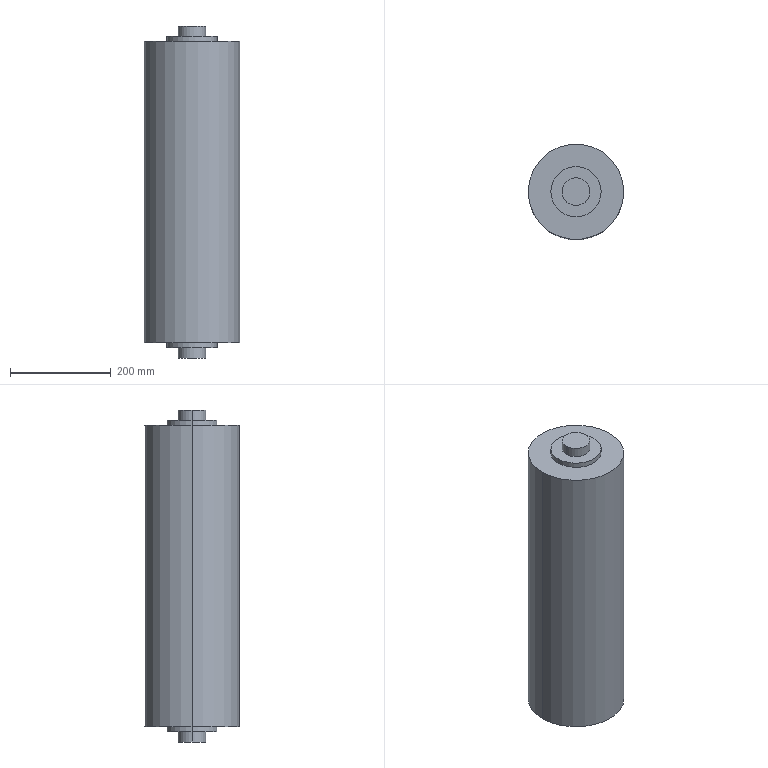Part | SolidWorks | features ICE 4, Extrusion 1 | 1 solid | 16 faces | box 190 x 190 x 660 mm | volume 17263837 mm3 | cylinder 10 | plane 6 | commonest cylinder face diameters 55 x4 100 x4 190 x2
STEP:
#1=CARTESIAN_POINT('',(27.5,0.,630.));
#2=VERTEX_POINT('',#1);
#3=CARTESIAN_POINT('',(-27.5,0.,630.));
#4=VERTEX_POINT('',#3);
#5=CARTESIAN_POINT('',(0.,0.,630.));
#6=DIRECTION('',(0.,0.,1.));
#7=DIRECTION('',(1.,0.,0.));
#8=AXIS2_PLACEMENT_3D('',#5,#6,#7);
#9=CIRCLE('',#8,27.5);
#10=EDGE_CURVE('',#2,#4,#9,.T.);
#11=ORIENTED_EDGE('',*,*,#10,.F.);
#12=CARTESIAN_POINT('',(27.5,0.,610.));
#13=VERTEX_POINT('',#12);
#14=CARTESIAN_POINT('',(27.5,0.,630.));
#15=DIRECTION('',(0.,0.,-1.));
#16=VECTOR('',#15,1000.);
#17=LINE('',#14,#16);
#18=EDGE_CURVE('',#2,#13,#17,.T.);
#19=ORIENTED_EDGE('',*,*,#18,.T.);
#20=CARTESIAN_POINT('',(-27.5,0.,610.));
#21=VERTEX_POINT('',#20);
#22=CARTESIAN_POINT('',(0.,0.,610.));
#23=DIRECTION('',(0.,0.,1.));
#24=DIRECTION('',(1.,0.,0.));
#25=AXIS2_PLACEMENT_3D('',#22,#23,#24);
#26=CIRCLE('',#25,27.5);
#27=EDGE_CURVE('',#13,#21,#26,.T.);
#28=ORIENTED_EDGE('',*,*,#27,.T.);
#29=CARTESIAN_POINT('',(-27.5,0.,630.));
#30=DIRECTION('',(0.,0.,-1.));
#31=VECTOR('',#30,1000.);
#32=LINE('',#29,#31);
#33=EDGE_CURVE('',#4,#21,#32,.T.);
#34=ORIENTED_EDGE('',*,*,#33,.F.);
#35=EDGE_LOOP('',(#11,#19,#28,#34));
#36=FACE_OUTER_BOUND('',#35,.T.);
#37=CARTESIAN_POINT('',(0.,0.,630.));
#38=DIRECTION('',(0.,0.,-1.));
#39=DIRECTION('',(-1.,0.,0.));
#40=AXIS2_PLACEMENT_3D('',#37,#38,#39);
#41=CYLINDRICAL_SURFACE('',#40,27.5);
#42=ADVANCED_FACE('',(#36),#41,.T.);
#43=CARTESIAN_POINT('',(-27.5,0.,-30.));
#44=VERTEX_POINT('',#43);
#45=CARTESIAN_POINT('',(27.5,0.,-30.));
#46=VERTEX_POINT('',#45);
#47=CARTESIAN_POINT('',(0.,0.,-30.));
#48=DIRECTION('',(0.,0.,-1.));
#49=DIRECTION('',(-1.,0.,0.));
#50=AXIS2_PLACEMENT_3D('',#47,#48,#49);
#51=CIRCLE('',#50,27.5);
#52=EDGE_CURVE('',#44,#46,#51,.T.);
#53=ORIENTED_EDGE('',*,*,#52,.F.);
#54=CARTESIAN_POINT('',(-27.5,0.,-10.));
#55=VERTEX_POINT('',#54);
#56=CARTESIAN_POINT('',(-27.5,0.,-30.));
#57=DIRECTION('',(0.,0.,1.));
#58=VECTOR('',#57,1000.);
#59=LINE('',#56,#58);
#60=EDGE_CURVE('',#44,#55,#59,.T.);
#61=ORIENTED_EDGE('',*,*,#60,.T.);
#62=CARTESIAN_POINT('',(27.5,0.,-10.));
#63=VERTEX_POINT('',#62);
#64=CARTESIAN_POINT('',(0.,0.,-10.));
#65=DIRECTION('',(0.,0.,-1.));
#66=DIRECTION('',(-1.,0.,0.));
#67=AXIS2_PLACEMENT_3D('',#64,#65,#66);
#68=CIRCLE('',#67,27.5);
#69=EDGE_CURVE('',#55,#63,#68,.T.);
#70=ORIENTED_EDGE('',*,*,#69,.T.);
#71=CARTESIAN_POINT('',(27.5,0.,-30.));
#72=DIRECTION('',(0.,0.,1.));
#73=VECTOR('',#72,1000.);
#74=LINE('',#71,#73);
#75=EDGE_CURVE('',#46,#63,#74,.T.);
#76=ORIENTED_EDGE('',*,*,#75,.F.);
#77=EDGE_LOOP('',(#53,#61,#70,#76));
#78=FACE_OUTER_BOUND('',#77,.T.);
#79=CARTESIAN_POINT('',(0.,0.,-30.));
#80=DIRECTION('',(0.,0.,1.));
#81=DIRECTION('',(1.,0.,0.));
#82=AXIS2_PLACEMENT_3D('',#79,#80,#81);
#83=CYLINDRICAL_SURFACE('',#82,27.5);
#84=ADVANCED_FACE('',(#78),#83,.T.);
#85=CARTESIAN_POINT('',(-50.,0.,-10.));
#86=VERTEX_POINT('',#85);
#87=CARTESIAN_POINT('',(50.,0.,-10.));
#88=VERTEX_POINT('',#87);
#89=CARTESIAN_POINT('',(0.,0.,-10.));
#90=DIRECTION('',(0.,0.,-1.));
#91=DIRECTION('',(-1.,0.,0.));
#92=AXIS2_PLACEMENT_3D('',#89,#90,#91);
#93=CIRCLE('',#92,50.);
#94=EDGE_CURVE('',#86,#88,#93,.T.);
#95=ORIENTED_EDGE('',*,*,#94,.F.);
#96=CARTESIAN_POINT('',(-50.,0.,0.));
#97=VERTEX_POINT('',#96);
#98=CARTESIAN_POINT('',(-50.,0.,-10.));
#99=DIRECTION('',(0.,0.,1.));
#100=VECTOR('',#99,1000.);
#101=LINE('',#98,#100);
#102=EDGE_CURVE('',#86,#97,#101,.T.);
#103=ORIENTED_EDGE('',*,*,#102,.T.);
#104=CARTESIAN_POINT('',(50.,0.,0.));
#105=VERTEX_POINT('',#104);
#106=CARTESIAN_POINT('',(0.,0.,0.));
#107=DIRECTION('',(0.,0.,-1.));
#108=DIRECTION('',(1.,0.,0.));
#109=AXIS2_PLACEMENT_3D('',#106,#107,#108);
#110=CIRCLE('',#109,50.);
#111=EDGE_CURVE('',#97,#105,#110,.T.);
#112=ORIENTED_EDGE('',*,*,#111,.T.);
#113=CARTESIAN_POINT('',(50.,0.,-10.));
#114=DIRECTION('',(0.,0.,1.));
#115=VECTOR('',#114,1000.);
#116=LINE('',#113,#115);
#117=EDGE_CURVE('',#88,#105,#116,.T.);
#118=ORIENTED_EDGE('',*,*,#117,.F.);
#119=EDGE_LOOP('',(#95,#103,#112,#118));
#120=FACE_OUTER_BOUND('',#119,.T.);
#121=CARTESIAN_POINT('',(0.,0.,-10.));
#122=DIRECTION('',(0.,0.,1.));
#123=DIRECTION('',(1.,0.,0.));
#124=AXIS2_PLACEMENT_3D('',#121,#122,#123);
#125=CYLINDRICAL_SURFACE('',#124,50.);
#126=ADVANCED_FACE('',(#120),#125,.T.);
#127=CARTESIAN_POINT('',(50.,0.,610.));
#128=VERTEX_POINT('',#127);
#129=CARTESIAN_POINT('',(-50.,0.,610.));
#130=VERTEX_POINT('',#129);
#131=CARTESIAN_POINT('',(0.,0.,610.));
#132=DIRECTION('',(0.,0.,1.));
#133=DIRECTION('',(1.,0.,0.));
#134=AXIS2_PLACEMENT_3D('',#131,#132,#133);
#135=CIRCLE('',#134,50.);
#136=EDGE_CURVE('',#128,#130,#135,.T.);
#137=ORIENTED_EDGE('',*,*,#136,.F.);
#138=CARTESIAN_POINT('',(50.,0.,600.));
#139=VERTEX_POINT('',#138);
#140=CARTESIAN_POINT('',(50.,0.,610.));
#141=DIRECTION('',(0.,0.,-1.));
#142=VECTOR('',#141,1000.);
#143=LINE('',#140,#142);
#144=EDGE_CURVE('',#128,#139,#143,.T.);
#145=ORIENTED_EDGE('',*,*,#144,.T.);
#146=CARTESIAN_POINT('',(-50.,0.,600.));
#147=VERTEX_POINT('',#146);
#148=CARTESIAN_POINT('',(0.,0.,600.));
#149=DIRECTION('',(0.,0.,1.));
#150=DIRECTION('',(1.,0.,0.));
#151=AXIS2_PLACEMENT_3D('',#148,#149,#150);
#152=CIRCLE('',#151,50.);
#153=EDGE_CURVE('',#139,#147,#152,.T.);
#154=ORIENTED_EDGE('',*,*,#153,.T.);
#155=CARTESIAN_POINT('',(-50.,0.,610.));
#156=DIRECTION('',(0.,0.,-1.));
#157=VECTOR('',#156,1000.);
#158=LINE('',#155,#157);
#159=EDGE_CURVE('',#130,#147,#158,.T.);
#160=ORIENTED_EDGE('',*,*,#159,.F.);
#161=EDGE_LOOP('',(#137,#145,#154,#160));
#162=FACE_OUTER_BOUND('',#161,.T.);
#163=CARTESIAN_POINT('',(0.,0.,610.));
#164=DIRECTION('',(0.,0.,-1.));
#165=DIRECTION('',(-1.,0.,0.));
#166=AXIS2_PLACEMENT_3D('',#163,#164,#165);
#167=CYLINDRICAL_SURFACE('',#166,50.);
#168=ADVANCED_FACE('',(#162),#167,.T.);
#169=CARTESIAN_POINT('',(95.,0.,600.));
#170=VERTEX_POINT('',#169);
#171=CARTESIAN_POINT('',(-95.,0.,600.));
#172=VERTEX_POINT('',#171);
#173=CARTESIAN_POINT('',(0.,0.,600.));
#174=DIRECTION('',(0.,0.,1.));
#175=DIRECTION('',(1.,0.,0.));
#176=AXIS2_PLACEMENT_3D('',#173,#174,#175);
#177=CIRCLE('',#176,95.);
#178=EDGE_CURVE('',#170,#172,#177,.T.);
#179=ORIENTED_EDGE('',*,*,#178,.F.);
#180=CARTESIAN_POINT('',(95.,0.,0.));
#181=VERTEX_POINT('',#180);
#182=CARTESIAN_POINT('',(95.,0.,600.));
#183=DIRECTION('',(0.,0.,-1.));
#184=VECTOR('',#183,1000.);
#185=LINE('',#182,#184);
#186=EDGE_CURVE('',#170,#181,#185,.T.);
#187=ORIENTED_EDGE('',*,*,#186,.T.);
#188=CARTESIAN_POINT('',(-95.,0.,0.));
#189=VERTEX_POINT('',#188);
#190=CARTESIAN_POINT('',(0.,0.,0.));
#191=DIRECTION('',(0.,0.,1.));
#192=DIRECTION('',(1.,0.,0.));
#193=AXIS2_PLACEMENT_3D('',#190,#191,#192);
#194=CIRCLE('',#193,95.);
#195=EDGE_CURVE('',#181,#189,#194,.T.);
#196=ORIENTED_EDGE('',*,*,#195,.T.);
#197=CARTESIAN_POINT('',(-95.,0.,600.));
#198=DIRECTION('',(0.,0.,-1.));
#199=VECTOR('',#198,1000.);
#200=LINE('',#197,#199);
#201=EDGE_CURVE('',#172,#189,#200,.T.);
#202=ORIENTED_EDGE('',*,*,#201,.F.);
#203=EDGE_LOOP('',(#179,#187,#196,#202));
#204=FACE_OUTER_BOUND('',#203,.T.);
#205=CARTESIAN_POINT('',(0.,0.,600.));
#206=DIRECTION('',(0.,0.,-1.));
#207=DIRECTION('',(-1.,0.,0.));
#208=AXIS2_PLACEMENT_3D('',#205,#206,#207);
#209=CYLINDRICAL_SURFACE('',#208,95.);
#210=ADVANCED_FACE('',(#204),#209,.T.);
#211=ORIENTED_EDGE('',*,*,#186,.F.);
#212=CARTESIAN_POINT('',(0.,0.,600.));
#213=DIRECTION('',(0.,0.,1.));
#214=DIRECTION('',(1.,0.,0.));
#215=AXIS2_PLACEMENT_3D('',#212,#213,#214);
#216=CIRCLE('',#215,95.);
#217=EDGE_CURVE('',#172,#170,#216,.T.);
#218=ORIENTED_EDGE('',*,*,#217,.F.);
#219=ORIENTED_EDGE('',*,*,#201,.T.);
#220=CARTESIAN_POINT('',(0.,0.,0.));
#221=DIRECTION('',(0.,0.,1.));
#222=DIRECTION('',(1.,0.,0.));
#223=AXIS2_PLACEMENT_3D('',#220,#221,#222);
#224=CIRCLE('',#223,95.);
#225=EDGE_CURVE('',#189,#181,#224,.T.);
#226=ORIENTED_EDGE('',*,*,#225,.T.);
#227=EDGE_LOOP('',(#211,#218,#219,#226));
#228=FACE_OUTER_BOUND('',#227,.T.);
#229=CARTESIAN_POINT('',(0.,0.,600.));
#230=DIRECTION('',(0.,0.,-1.));
#231=DIRECTION('',(-1.,0.,0.));
#232=AXIS2_PLACEMENT_3D('',#229,#230,#231);
#233=CYLINDRICAL_SURFACE('',#232,95.);
#234=ADVANCED_FACE('',(#228),#233,.T.);
#235=CARTESIAN_POINT('',(0.,0.,600.));
#236=DIRECTION('',(0.,0.,1.));
#237=DIRECTION('',(1.,0.,0.));
#238=AXIS2_PLACEMENT_3D('',#235,#236,#237);
#239=CIRCLE('',#238,50.);
#240=EDGE_CURVE('',#147,#139,#239,.T.);
#241=ORIENTED_EDGE('',*,*,#240,.F.);
#242=ORIENTED_EDGE('',*,*,#153,.F.);
#243=EDGE_LOOP('',(#241,#242));
#244=FACE_BOUND('',#243,.T.);
#245=ORIENTED_EDGE('',*,*,#217,.T.);
#246=ORIENTED_EDGE('',*,*,#178,.T.);
#247=EDGE_LOOP('',(#245,#246));
#248=FACE_OUTER_BOUND('',#247,.T.);
#249=CARTESIAN_POINT('',(0.,0.,600.));
#250=DIRECTION('',(0.,0.,1.));
#251=DIRECTION('',(1.,0.,0.));
#252=AXIS2_PLACEMENT_3D('',#249,#250,#251);
#253=PLANE('',#252);
#254=ADVANCED_FACE('',(#244,#248),#253,.T.);
#255=CARTESIAN_POINT('',(0.,0.,0.));
#256=DIRECTION('',(0.,0.,-1.));
#257=DIRECTION('',(1.,0.,0.));
#258=AXIS2_PLACEMENT_3D('',#255,#256,#257);
#259=CIRCLE('',#258,50.);
#260=EDGE_CURVE('',#105,#97,#259,.T.);
#261=ORIENTED_EDGE('',*,*,#260,.F.);
#262=ORIENTED_EDGE('',*,*,#111,.F.);
#263=EDGE_LOOP('',(#261,#262));
#264=FACE_BOUND('',#263,.T.);
#265=ORIENTED_EDGE('',*,*,#225,.F.);
#266=ORIENTED_EDGE('',*,*,#195,.F.);
#267=EDGE_LOOP('',(#265,#266));
#268=FACE_OUTER_BOUND('',#267,.T.);
#269=CARTESIAN_POINT('',(0.,0.,0.));
#270=DIRECTION('',(0.,0.,1.));
#271=DIRECTION('',(1.,0.,0.));
#272=AXIS2_PLACEMENT_3D('',#269,#270,#271);
#273=PLANE('',#272);
#274=ADVANCED_FACE('',(#264,#268),#273,.F.);
#275=ORIENTED_EDGE('',*,*,#144,.F.);
#276=CARTESIAN_POINT('',(0.,0.,610.));
#277=DIRECTION('',(0.,0.,1.));
#278=DIRECTION('',(1.,0.,0.));
#279=AXIS2_PLACEMENT_3D('',#276,#277,#278);
#280=CIRCLE('',#279,50.);
#281=EDGE_CURVE('',#130,#128,#280,.T.);
#282=ORIENTED_EDGE('',*,*,#281,.F.);
#283=ORIENTED_EDGE('',*,*,#159,.T.);
#284=ORIENTED_EDGE('',*,*,#240,.T.);
#285=EDGE_LOOP('',(#275,#282,#283,#284));
#286=FACE_OUTER_BOUND('',#285,.T.);
#287=CARTESIAN_POINT('',(0.,0.,610.));
#288=DIRECTION('',(0.,0.,-1.));
#289=DIRECTION('',(-1.,0.,0.));
#290=AXIS2_PLACEMENT_3D('',#287,#288,#289);
#291=CYLINDRICAL_SURFACE('',#290,50.);
#292=ADVANCED_FACE('',(#286),#291,.T.);
#293=CARTESIAN_POINT('',(0.,0.,610.));
#294=DIRECTION('',(0.,0.,1.));
#295=DIRECTION('',(1.,0.,0.));
#296=AXIS2_PLACEMENT_3D('',#293,#294,#295);
#297=CIRCLE('',#296,27.5);
#298=EDGE_CURVE('',#21,#13,#297,.T.);
#299=ORIENTED_EDGE('',*,*,#298,.F.);
#300=ORIENTED_EDGE('',*,*,#27,.F.);
#301=EDGE_LOOP('',(#299,#300));
#302=FACE_BOUND('',#301,.T.);
#303=ORIENTED_EDGE('',*,*,#281,.T.);
#304=ORIENTED_EDGE('',*,*,#136,.T.);
#305=EDGE_LOOP('',(#303,#304));
#306=FACE_OUTER_BOUND('',#305,.T.);
#307=CARTESIAN_POINT('',(0.,0.,610.));
#308=DIRECTION('',(0.,0.,1.));
#309=DIRECTION('',(1.,0.,0.));
#310=AXIS2_PLACEMENT_3D('',#307,#308,#309);
#311=PLANE('',#310);
#312=ADVANCED_FACE('',(#302,#306),#311,.T.);
#313=ORIENTED_EDGE('',*,*,#102,.F.);
#314=CARTESIAN_POINT('',(0.,0.,-10.));
#315=DIRECTION('',(0.,0.,-1.));
#316=DIRECTION('',(-1.,0.,0.));
#317=AXIS2_PLACEMENT_3D('',#314,#315,#316);
#318=CIRCLE('',#317,50.);
#319=EDGE_CURVE('',#88,#86,#318,.T.);
#320=ORIENTED_EDGE('',*,*,#319,.F.);
#321=ORIENTED_EDGE('',*,*,#117,.T.);
#322=ORIENTED_EDGE('',*,*,#260,.T.);
#323=EDGE_LOOP('',(#313,#320,#321,#322));
#324=FACE_OUTER_BOUND('',#323,.T.);
#325=CARTESIAN_POINT('',(0.,0.,-10.));
#326=DIRECTION('',(0.,0.,1.));
#327=DIRECTION('',(1.,0.,0.));
#328=AXIS2_PLACEMENT_3D('',#325,#326,#327);
#329=CYLINDRICAL_SURFACE('',#328,50.);
#330=ADVANCED_FACE('',(#324),#329,.T.);
#331=CARTESIAN_POINT('',(0.,0.,-10.));
#332=DIRECTION('',(0.,0.,-1.));
#333=DIRECTION('',(-1.,0.,0.));
#334=AXIS2_PLACEMENT_3D('',#331,#332,#333);
#335=CIRCLE('',#334,27.5);
#336=EDGE_CURVE('',#63,#55,#335,.T.);
#337=ORIENTED_EDGE('',*,*,#336,.F.);
#338=ORIENTED_EDGE('',*,*,#69,.F.);
#339=EDGE_LOOP('',(#337,#338));
#340=FACE_BOUND('',#339,.T.);
#341=ORIENTED_EDGE('',*,*,#319,.T.);
#342=ORIENTED_EDGE('',*,*,#94,.T.);
#343=EDGE_LOOP('',(#341,#342));
#344=FACE_OUTER_BOUND('',#343,.T.);
#345=CARTESIAN_POINT('',(0.,0.,-10.));
#346=DIRECTION('',(0.,0.,-1.));
#347=DIRECTION('',(-1.,0.,0.));
#348=AXIS2_PLACEMENT_3D('',#345,#346,#347);
#349=PLANE('',#348);
#350=ADVANCED_FACE('',(#340,#344),#349,.T.);
#351=ORIENTED_EDGE('',*,*,#60,.F.);
#352=CARTESIAN_POINT('',(0.,0.,-30.));
#353=DIRECTION('',(0.,0.,-1.));
#354=DIRECTION('',(-1.,0.,0.));
#355=AXIS2_PLACEMENT_3D('',#352,#353,#354);
#356=CIRCLE('',#355,27.5);
#357=EDGE_CURVE('',#46,#44,#356,.T.);
#358=ORIENTED_EDGE('',*,*,#357,.F.);
#359=ORIENTED_EDGE('',*,*,#75,.T.);
#360=ORIENTED_EDGE('',*,*,#336,.T.);
#361=EDGE_LOOP('',(#351,#358,#359,#360));
#362=FACE_OUTER_BOUND('',#361,.T.);
#363=CARTESIAN_POINT('',(0.,0.,-30.));
#364=DIRECTION('',(0.,0.,1.));
#365=DIRECTION('',(1.,0.,0.));
#366=AXIS2_PLACEMENT_3D('',#363,#364,#365);
#367=CYLINDRICAL_SURFACE('',#366,27.5);
#368=ADVANCED_FACE('',(#362),#367,.T.);
#369=ORIENTED_EDGE('',*,*,#357,.T.);
#370=ORIENTED_EDGE('',*,*,#52,.T.);
#371=EDGE_LOOP('',(#369,#370));
#372=FACE_OUTER_BOUND('',#371,.T.);
#373=CARTESIAN_POINT('',(0.,0.,-30.));
#374=DIRECTION('',(0.,0.,-1.));
#375=DIRECTION('',(-1.,0.,0.));
#376=AXIS2_PLACEMENT_3D('',#373,#374,#375);
#377=PLANE('',#376);
#378=ADVANCED_FACE('',(#372),#377,.T.);
#379=ORIENTED_EDGE('',*,*,#18,.F.);
#380=CARTESIAN_POINT('',(0.,0.,630.));
#381=DIRECTION('',(0.,0.,1.));
#382=DIRECTION('',(1.,0.,0.));
#383=AXIS2_PLACEMENT_3D('',#380,#381,#382);
#384=CIRCLE('',#383,27.5);
#385=EDGE_CURVE('',#4,#2,#384,.T.);
#386=ORIENTED_EDGE('',*,*,#385,.F.);
#387=ORIENTED_EDGE('',*,*,#33,.T.);
#388=ORIENTED_EDGE('',*,*,#298,.T.);
#389=EDGE_LOOP('',(#379,#386,#387,#388));
#390=FACE_OUTER_BOUND('',#389,.T.);
#391=CARTESIAN_POINT('',(0.,0.,630.));
#392=DIRECTION('',(0.,0.,-1.));
#393=DIRECTION('',(-1.,0.,0.));
#394=AXIS2_PLACEMENT_3D('',#391,#392,#393);
#395=CYLINDRICAL_SURFACE('',#394,27.5);
#396=ADVANCED_FACE('',(#390),#395,.T.);
#397=ORIENTED_EDGE('',*,*,#385,.T.);
#398=ORIENTED_EDGE('',*,*,#10,.T.);
#399=EDGE_LOOP('',(#397,#398));
#400=FACE_OUTER_BOUND('',#399,.T.);
#401=CARTESIAN_POINT('',(0.,0.,630.));
#402=DIRECTION('',(0.,0.,1.));
#403=DIRECTION('',(1.,0.,0.));
#404=AXIS2_PLACEMENT_3D('',#401,#402,#403);
#405=PLANE('',#404);
#406=ADVANCED_FACE('',(#400),#405,.T.);
#407=CLOSED_SHELL('',(#42,#84,#126,#168,#210,#234,#254,#274,#292,#312,#330,#350,#368,#378,#396,#406));
#408=MANIFOLD_SOLID_BREP('',#407);
#409=CARTESIAN_POINT('',(0.,0.,0.));
#410=DIRECTION('',(0.,0.,1.));
#411=DIRECTION('',(1.,0.,0.));
#412=AXIS2_PLACEMENT_3D('',#409,#410,#411);
#413=(LENGTH_UNIT()NAMED_UNIT(*)SI_UNIT(.MILLI.,.METRE.));
#414=UNCERTAINTY_MEASURE_WITH_UNIT(LENGTH_MEASURE(0.00001),#413,'','');
#415=(NAMED_UNIT(*)PLANE_ANGLE_UNIT()SI_UNIT($,.RADIAN.));
#416=(NAMED_UNIT(*)SI_UNIT($,.STERADIAN.)SOLID_ANGLE_UNIT());
#417=(GEOMETRIC_REPRESENTATION_CONTEXT(3)GLOBAL_UNCERTAINTY_ASSIGNED_CONTEXT((#414))GLOBAL_UNIT_ASSIGNED_CONTEXT((#413,#415,#416))REPRESENTATION_CONTEXT('',''));
#418=ADVANCED_BREP_SHAPE_REPRESENTATION('',(#408,#412),#417);